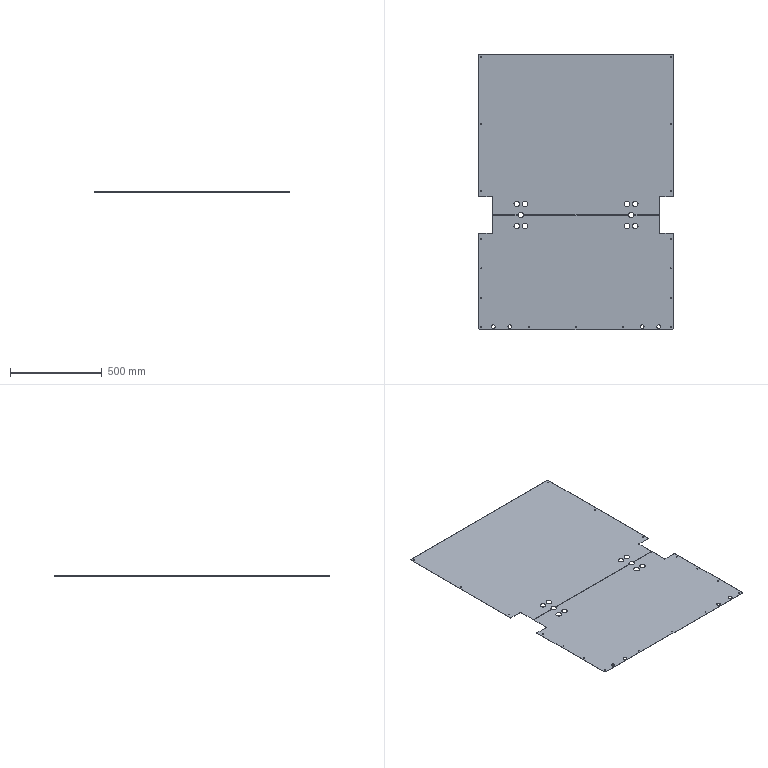Part | SolidWorks | features ICE 4, FlatPattern 2, Cut 1, Fillet 1, MirrorPattern 1, SMBaseFlange 1, SheetMetal 1 | 2 solids | 88 faces | box 1060 x 1500 x 1 mm | volume 1549579 mm3 | cylinder 64 | plane 24 | commonest cylinder face diameters 5 x34 30 x20 20 x8 24 x2